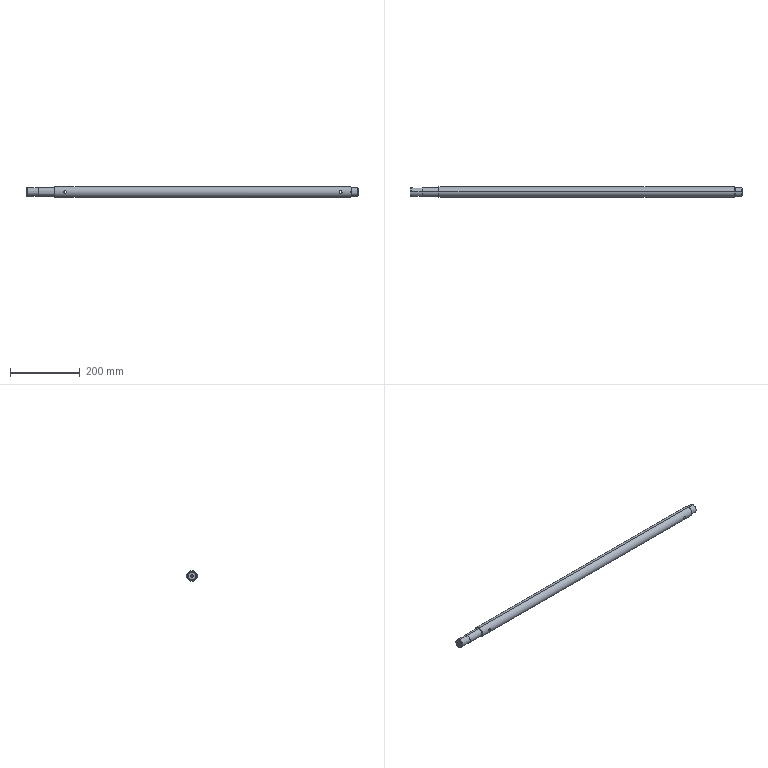Part | SolidWorks | features BaseBody 1 | 1 solid | 42 faces | box 955.3 x 30 x 30 mm | volume 646249 mm3 | cylinder 21 | plane 11 | cone 10 | commonest cylinder face diameters 8 x7 24 x4 25 x4 6.647 x2 22 x2 30 x2